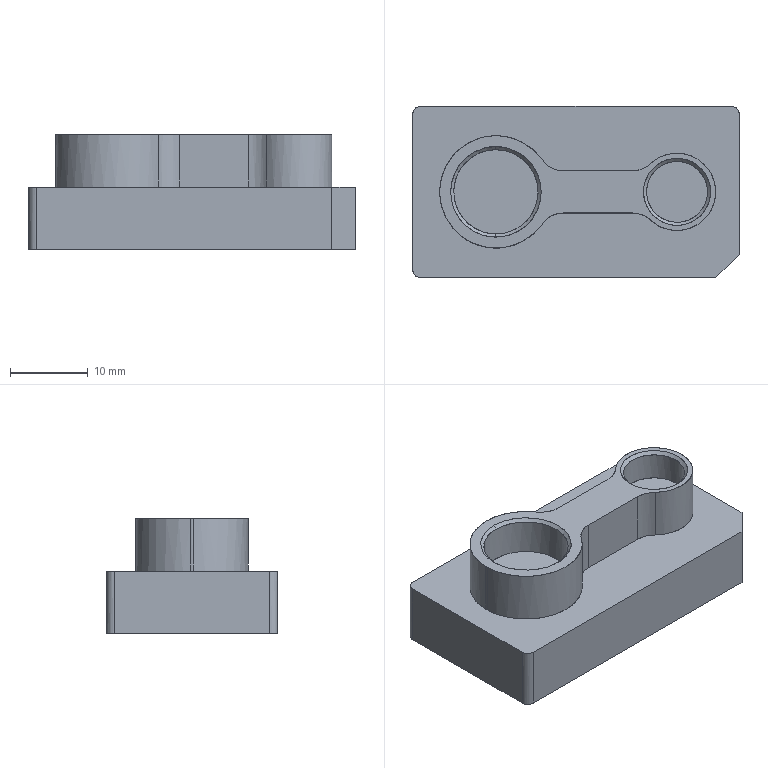NC program | PowerMill | posted by the shop | part box 42 x 22 x 14.721 mm
Lines 1 to 1508 of 84704:
%
G40 G49 G17 G80
( TOOL ID   D10C_1_1 )
( TOOL DIA. 10. TIP RAD 0 LENGTH 70.16 )
( Z = -.069 )
T1 M6
T2
G91 G28 Z0
G0 G90 G54
M08
S8000 M3
G0 X0 Y0 M8
G43 Z10.2 H1
X28.78 Y13.78
Z1.131
G1 Z-.069 F6000
X23.78 F10000
X-23.78
Y8.268
X23.78
Y2.756
X-23.78
Y-2.756
X23.78
Y-8.268
X-23.78
Y-13.78
X23.78
X28.78
G0 Z10.2
X.211 Y.009
Z9.881
X31.026 Y4.95
Z.692
G1 Z-.508 F6000
X30.499 F10000
G3 X25.751 Y.202 I0 J-4.747
G1 Y-14.007
G2 X24.751 Y-15.007 I-1. J0
G1 X-24.329
G2 X-25.329 Y-14.007 I0 J1.
G1 Y14.024
G2 X-24.329 Y15.024 I1. J0
G1 X24.751
G2 X25.751 Y14.024 I0 J-1.
G1 Y.202
X23.249 Y.105
X23.253 Y.009
X23.224 Y-.765
X23.136 Y-1.538
X22.988 Y-2.312
X22.777 Y-3.085
X22.497 Y-3.859
X22.147 Y-4.632
X21.867 Y-5.145
X21.182 Y-6.179
X20.32 Y-7.179
X19.547 Y-7.885
X18.773 Y-8.463
X18. Y-8.949
X17.226 Y-9.333
X16.453 Y-9.653
X15.68 Y-9.894
X15.033 Y-10.046
X14.133 Y-10.189
X13.359 Y-10.245
X12.586 Y-10.243
X11.812 Y-10.182
X11.039 Y-10.063
X10.266 Y-9.879
X9.492 Y-9.634
X8.719 Y-9.315
X7.945 Y-8.916
X7.266 Y-8.499
X6.727 Y-8.093
X6.585 Y-8.019
X6.427 Y-7.993
X-.452
G3 X-.828 Y-8.163 I0 J-.5
G1 X-1.123 Y-8.499
X-1.91 Y-9.273
X-2.849 Y-10.046
X-3.656 Y-10.599
X-4.029 Y-10.819
X-5.203 Y-11.421
X-5.976 Y-11.737
X-6.75 Y-11.987
X-7.523 Y-12.2
X-8.443 Y-12.366
X-9.07 Y-12.45
X-9.844 Y-12.499
X-10.617 Y-12.506
X-11.39 Y-12.465
X-12.164 Y-12.371
X-12.937 Y-12.23
X-13.711 Y-12.037
X-15.012 Y-11.593
X-16.031 Y-11.122
X-16.584 Y-10.819
X-17.578 Y-10.177
X-18.351 Y-9.581
X-18.696 Y-9.273
X-19.487 Y-8.499
X-20.144 Y-7.726
X-20.672 Y-6.988
X-21.185 Y-6.179
X-21.588 Y-5.405
X-21.925 Y-4.632
X-22.206 Y-3.859
X-22.427 Y-3.085
X-22.594 Y-2.312
X-22.722 Y-1.538
X-22.83 Y.009
X-22.719 Y1.555
X-22.594 Y2.329
X-22.421 Y3.102
X-22.218 Y3.825
X-21.917 Y4.649
X-21.572 Y5.422
X-21.175 Y6.196
X-20.687 Y6.969
X-20.133 Y7.743
X-19.469 Y8.516
X-18.687 Y9.29
X-17.739 Y10.063
X-16.56 Y10.836
X-15.258 Y11.491
X-14.961 Y11.61
X-13.711 Y12.04
X-12.937 Y12.233
X-12.099 Y12.383
X-10.617 Y12.516
X-9.844 Y12.505
X-8.511 Y12.383
X-7.523 Y12.2
X-6.75 Y11.989
X-5.639 Y11.61
X-4.43 Y11.048
X-3.656 Y10.598
X-2.883 Y10.071
X-2.109 Y9.454
X-1.336 Y8.712
X-.829 Y8.156
G3 X-.46 Y7.993 I.37 J.337
G1 X6.424
X6.584 Y8.019
X6.727 Y8.095
X7.172 Y8.435
X7.945 Y8.916
X8.663 Y9.29
X9.492 Y9.634
X10.266 Y9.879
X11.04 Y10.063
X11.812 Y10.182
X12.586 Y10.243
X13.359 Y10.245
X14.133 Y10.188
X14.906 Y10.073
X15.68 Y9.894
X16.453 Y9.653
X17.226 Y9.333
X18. Y8.949
X18.773 Y8.463
X19.547 Y7.885
X20.32 Y7.179
X21.094 Y6.292
X21.69 Y5.422
X22.138 Y4.649
X22.49 Y3.876
X22.772 Y3.102
X22.984 Y2.329
X23.134 Y1.555
X23.223 Y.782
X23.249 Y.105
X25.751 Y.202
G0 Z3.303
G1 X31.026 Y4.95
G0 Z.303
G1 Z-.897 F6000
X30.499 F10000
G3 X25.751 Y.202 I0 J-4.747
G1 Y-14.007
G2 X24.751 Y-15.007 I-1. J0
G1 X-24.329
G2 X-25.329 Y-14.007 I0 J1.
G1 Y14.024
G2 X-24.329 Y15.024 I1. J0
G1 X24.751
G2 X25.751 Y14.024 I0 J-1.
G1 Y.202
X23.249 Y.105
X23.253 Y.009
X23.224 Y-.765
X23.137 Y-1.538
X22.988 Y-2.312
X22.777 Y-3.085
X22.497 Y-3.859
X22.147 Y-4.632
X21.867 Y-5.145
X21.182 Y-6.179
X20.32 Y-7.179
X19.547 Y-7.885
X18.773 Y-8.463
X18. Y-8.949
X17.226 Y-9.333
X16.453 Y-9.653
X15.68 Y-9.894
X15.033 Y-10.046
X14.133 Y-10.189
X13.359 Y-10.245
X12.586 Y-10.243
X11.812 Y-10.182
X11.039 Y-10.063
X10.266 Y-9.879
X9.492 Y-9.634
X8.719 Y-9.315
X7.945 Y-8.916
X7.266 Y-8.499
X6.727 Y-8.093
X6.585 Y-8.019
X6.427 Y-7.993
X-.452
G3 X-.828 Y-8.163 I0 J-.5
G1 X-1.123 Y-8.499
X-1.91 Y-9.273
X-2.849 Y-10.046
X-3.656 Y-10.599
X-4.029 Y-10.819
X-5.203 Y-11.421
X-5.976 Y-11.737
X-6.75 Y-11.987
X-7.523 Y-12.2
X-8.443 Y-12.366
X-9.07 Y-12.45
X-9.844 Y-12.499
X-10.617 Y-12.506
X-11.39 Y-12.465
X-12.164 Y-12.371
X-12.937 Y-12.23
X-13.711 Y-12.037
X-15.012 Y-11.593
X-16.031 Y-11.122
X-16.584 Y-10.819
X-17.578 Y-10.177
X-18.351 Y-9.581
X-18.696 Y-9.273
X-19.487 Y-8.499
X-20.144 Y-7.726
X-20.672 Y-6.988
X-21.185 Y-6.179
X-21.588 Y-5.405
X-21.925 Y-4.632
X-22.206 Y-3.859
X-22.427 Y-3.085
X-22.594 Y-2.312
X-22.722 Y-1.538
X-22.83 Y.009
X-22.719 Y1.555
X-22.594 Y2.329
X-22.421 Y3.102
X-22.218 Y3.825
X-21.917 Y4.649
X-21.572 Y5.422
X-21.176 Y6.196
X-20.687 Y6.969
X-20.133 Y7.743
X-19.469 Y8.516
X-18.687 Y9.29
X-17.739 Y10.063
X-16.56 Y10.836
X-15.258 Y11.491
X-14.961 Y11.61
X-13.711 Y12.04
X-12.937 Y12.233
X-12.099 Y12.383
X-10.617 Y12.516
X-9.844 Y12.505
X-8.511 Y12.383
X-7.523 Y12.2
X-6.75 Y11.989
X-5.639 Y11.61
X-4.43 Y11.048
X-3.656 Y10.598
X-2.883 Y10.071
X-2.109 Y9.454
X-1.336 Y8.712
X-.829 Y8.156
G3 X-.46 Y7.993 I.37 J.337
G1 X6.424
X6.584 Y8.019
X6.727 Y8.095
X7.172 Y8.435
X7.945 Y8.916
X8.663 Y9.29
X9.492 Y9.634
X10.266 Y9.879
X11.04 Y10.063
X11.812 Y10.182
X12.586 Y10.243
X13.359 Y10.245
X14.133 Y10.188
X14.906 Y10.073
X15.68 Y9.894
X16.453 Y9.653
X17.226 Y9.333
X18. Y8.949
X18.773 Y8.463
X19.547 Y7.885
X20.32 Y7.179
X21.094 Y6.292
X21.69 Y5.422
X22.138 Y4.649
X22.49 Y3.876
X22.772 Y3.102
X22.984 Y2.329
X23.134 Y1.555
X23.223 Y.782
X23.249 Y.105
X25.751 Y.202
G0 Z2.914
G1 X31.026 Y4.95
G0 Z-.086
G1 Z-1.286 F6000
X30.499 F10000
G3 X25.751 Y.202 I0 J-4.747
G1 Y-14.007
G2 X24.751 Y-15.007 I-1. J0
G1 X-24.329
G2 X-25.329 Y-14.007 I0 J1.
G1 Y14.024
G2 X-24.329 Y15.024 I1. J0
G1 X24.751
G2 X25.751 Y14.024 I0 J-1.
G1 Y.202
X23.249 Y.105
X23.253 Y.009
X23.224 Y-.765
X23.137 Y-1.538
X22.988 Y-2.312
X22.777 Y-3.085
X22.497 Y-3.859
X22.147 Y-4.632
X21.867 Y-5.145
X21.182 Y-6.179
X20.32 Y-7.179
X19.547 Y-7.885
X18.773 Y-8.463
X18. Y-8.949
X17.226 Y-9.333
X16.453 Y-9.653
X15.68 Y-9.894
X15.664 Y-9.897
X15.033 Y-10.046
X15.002 Y-10.051
X14.906 Y-10.073
X14.133 Y-10.189
X13.359 Y-10.245
X12.586 Y-10.243
X11.812 Y-10.182
X11.039 Y-10.063
X10.266 Y-9.879
X9.492 Y-9.634
X8.719 Y-9.315
X7.945 Y-8.916
X7.266 Y-8.499
X6.727 Y-8.093
X6.585 Y-8.019
X6.427 Y-7.993
X-.452
G3 X-.828 Y-8.163 I0 J-.5
G1 X-1.123 Y-8.499
X-1.91 Y-9.273
X-2.849 Y-10.046
X-3.656 Y-10.599
X-4.029 Y-10.819
X-5.203 Y-11.421
X-5.976 Y-11.737
X-6.75 Y-11.987
X-7.523 Y-12.2
X-8.443 Y-12.366
X-9.07 Y-12.45
X-9.844 Y-12.499
X-10.617 Y-12.506
X-11.39 Y-12.465
X-12.164 Y-12.371
X-12.937 Y-12.23
X-13.711 Y-12.037
X-15.012 Y-11.593
X-16.031 Y-11.122
X-16.584 Y-10.819
X-17.578 Y-10.177
X-18.351 Y-9.581
X-18.696 Y-9.273
X-19.487 Y-8.499
X-20.144 Y-7.726
X-20.672 Y-6.988
X-21.185 Y-6.179
X-21.588 Y-5.405
X-21.925 Y-4.632
X-22.206 Y-3.859
X-22.427 Y-3.085
X-22.594 Y-2.312
X-22.722 Y-1.538
X-22.83 Y.009
X-22.719 Y1.555
X-22.594 Y2.329
X-22.421 Y3.102
X-22.218 Y3.825
X-21.917 Y4.649
X-21.572 Y5.422
X-21.176 Y6.196
X-20.687 Y6.969
X-20.133 Y7.743
X-19.469 Y8.516
X-18.687 Y9.29
X-17.739 Y10.063
X-16.56 Y10.836
X-15.258 Y11.491
X-14.961 Y11.61
X-13.711 Y12.04
X-12.937 Y12.233
X-12.099 Y12.383
X-10.617 Y12.516
X-9.844 Y12.505
X-8.511 Y12.383
X-7.523 Y12.2
X-6.75 Y11.989
X-5.639 Y11.61
X-4.43 Y11.048
X-3.656 Y10.598
X-2.883 Y10.071
X-2.109 Y9.454
X-1.336 Y8.712
X-.829 Y8.156
G3 X-.46 Y7.993 I.37 J.337
G1 X6.424
X6.584 Y8.019
X6.727 Y8.095
X7.172 Y8.435
X7.945 Y8.916
X8.663 Y9.29
X9.492 Y9.634
X10.266 Y9.879
X11.04 Y10.063
X11.812 Y10.182
X12.586 Y10.243
X13.359 Y10.245
X14.133 Y10.188
X14.906 Y10.073
X15.68 Y9.894
X16.453 Y9.653
X17.226 Y9.333
X18. Y8.949
X18.773 Y8.463
X19.547 Y7.885
X20.32 Y7.179
X21.094 Y6.292
X21.69 Y5.422
X22.138 Y4.649
X22.49 Y3.876
X22.772 Y3.102
X22.984 Y2.329
X23.134 Y1.555
X23.223 Y.782
X23.249 Y.105
X25.751 Y.202
G0 Z2.525
G1 X31.026 Y4.95
G0 Z-.475
G1 Z-1.675 F6000
X30.499 F10000
G3 X25.751 Y.202 I0 J-4.747
G1 Y-14.007
G2 X24.751 Y-15.007 I-1. J0
G1 X-24.329
G2 X-25.329 Y-14.007 I0 J1.
G1 Y14.024
G2 X-24.329 Y15.024 I1. J0
G1 X24.751
G2 X25.751 Y14.024 I0 J-1.
G1 Y.202
X23.249 Y.105
X23.253 Y.009
X23.224 Y-.765
X23.137 Y-1.538
X22.988 Y-2.312
X22.777 Y-3.085
X22.497 Y-3.859
X22.147 Y-4.632
X21.867 Y-5.145
X21.182 Y-6.179
X20.32 Y-7.179
X19.547 Y-7.885
X18.773 Y-8.463
X18. Y-8.949
X17.226 Y-9.333
X16.453 Y-9.653
X15.68 Y-9.894
X15.648 Y-9.901
X15.033 Y-10.046
X15.003 Y-10.051
X14.906 Y-10.073
X14.133 Y-10.189
X13.359 Y-10.245
X12.586 Y-10.243
X11.812 Y-10.182
X11.039 Y-10.063
X10.266 Y-9.879
X9.492 Y-9.634
X8.719 Y-9.315
X7.945 Y-8.916
X7.266 Y-8.499
X6.727 Y-8.093
X6.585 Y-8.019
X6.427 Y-7.993
X-.452
G3 X-.828 Y-8.163 I0 J-.5
G1 X-1.123 Y-8.499
X-1.91 Y-9.273
X-2.849 Y-10.046
X-3.656 Y-10.599
X-4.029 Y-10.819
X-5.203 Y-11.421
X-5.976 Y-11.737
X-6.75 Y-11.987
X-7.523 Y-12.2
X-8.443 Y-12.366
X-9.07 Y-12.45
X-9.844 Y-12.499
X-10.617 Y-12.506
X-11.39 Y-12.465
X-12.164 Y-12.371
X-12.937 Y-12.23
X-13.711 Y-12.037
X-15.012 Y-11.593
X-16.031 Y-11.122
X-16.584 Y-10.819
X-17.578 Y-10.178
X-18.351 Y-9.581
X-18.696 Y-9.273
X-19.487 Y-8.499
X-20.144 Y-7.726
X-20.672 Y-6.988
X-21.185 Y-6.179
X-21.588 Y-5.405
X-21.925 Y-4.632
X-22.206 Y-3.859
X-22.427 Y-3.085
X-22.594 Y-2.312
X-22.722 Y-1.538
X-22.83 Y.009
X-22.719 Y1.555
X-22.594 Y2.329
X-22.421 Y3.102
X-22.218 Y3.825
X-21.917 Y4.649
X-21.572 Y5.422
X-21.176 Y6.196
X-20.687 Y6.969
X-20.133 Y7.743
X-19.469 Y8.516
X-18.687 Y9.29
X-17.739 Y10.063
X-16.56 Y10.836
X-15.258 Y11.491
X-14.961 Y11.61
X-13.711 Y12.04
X-12.937 Y12.233
X-12.099 Y12.383
X-10.617 Y12.516
X-9.844 Y12.505
X-8.511 Y12.383
X-7.523 Y12.2
X-6.75 Y11.989
X-5.639 Y11.61
X-4.43 Y11.048
X-3.656 Y10.598
X-2.883 Y10.071
X-2.109 Y9.454
X-1.336 Y8.712
X-.829 Y8.156
G3 X-.46 Y7.993 I.37 J.337
G1 X6.424
X6.584 Y8.019
X6.727 Y8.095
X7.172 Y8.435
X7.945 Y8.916
X8.663 Y9.29
X9.492 Y9.634
X10.266 Y9.879
X11.04 Y10.063
X11.812 Y10.182
X12.586 Y10.243
X13.359 Y10.245
X14.133 Y10.188
X14.906 Y10.073
X15.68 Y9.894
X16.453 Y9.653
X17.226 Y9.333
X18. Y8.949
X18.773 Y8.463
X19.547 Y7.885
X20.32 Y7.179
X21.094 Y6.292
X21.69 Y5.422
X22.138 Y4.649
X22.49 Y3.876
X22.772 Y3.102
X22.984 Y2.329
X23.134 Y1.555
X23.223 Y.782
X23.249 Y.105
X25.751 Y.202
G0 Z2.137
G1 X31.026 Y4.95
G0 Z-.863
G1 Z-2.063 F6000
X30.499 F10000
G3 X25.751 Y.202 I0 J-4.747
G1 Y-14.007
G2 X24.751 Y-15.007 I-1. J0
G1 X-24.329
G2 X-25.329 Y-14.007 I0 J1.
G1 Y14.024
G2 X-24.329 Y15.024 I1. J0
G1 X24.751
G2 X25.751 Y14.024 I0 J-1.
G1 Y.202
X23.249 Y.105
X23.253 Y.009
X23.224 Y-.765
X23.137 Y-1.538
X22.988 Y-2.312
X22.777 Y-3.085
X22.497 Y-3.859
X22.147 Y-4.632
X21.867 Y-5.145
X21.182 Y-6.179
X20.32 Y-7.179
X19.547 Y-7.885
X18.773 Y-8.463
X18. Y-8.949
X17.226 Y-9.333
X16.453 Y-9.653
X15.68 Y-9.894
X15.632 Y-9.905
X15.033 Y-10.046
X15.004 Y-10.05
X14.906 Y-10.073
X14.133 Y-10.189
X13.359 Y-10.245
X12.586 Y-10.243
X11.812 Y-10.182
X11.039 Y-10.063
X10.266 Y-9.879
X9.492 Y-9.634
X8.719 Y-9.315
X7.945 Y-8.916
X7.266 Y-8.499
X6.727 Y-8.093
X6.585 Y-8.019
X6.427 Y-7.993
X-.452
G3 X-.828 Y-8.163 I0 J-.5
G1 X-1.123 Y-8.499
X-1.91 Y-9.273
X-2.849 Y-10.046
X-3.656 Y-10.599
X-4.029 Y-10.819
X-5.203 Y-11.421
X-5.976 Y-11.737
X-6.75 Y-11.987
X-7.523 Y-12.2
X-8.443 Y-12.366
X-9.07 Y-12.45
X-9.844 Y-12.499
X-10.617 Y-12.506
X-11.39 Y-12.465
X-12.164 Y-12.371
X-12.937 Y-12.23
X-13.711 Y-12.037
X-15.012 Y-11.593
X-16.031 Y-11.122
X-16.584 Y-10.819
X-17.578 Y-10.178
X-18.351 Y-9.581
X-18.696 Y-9.273
X-19.487 Y-8.499
X-20.144 Y-7.726
X-20.672 Y-6.988
X-21.185 Y-6.179
X-21.588 Y-5.405
X-21.925 Y-4.632
X-22.206 Y-3.859
X-22.427 Y-3.085
X-22.594 Y-2.312
X-22.722 Y-1.538
X-22.83 Y.009
X-22.719 Y1.555
X-22.594 Y2.329
X-22.421 Y3.102
X-22.218 Y3.825
X-21.917 Y4.649
X-21.572 Y5.422
X-21.176 Y6.196
X-20.687 Y6.969
X-20.133 Y7.743
X-19.469 Y8.516
X-18.687 Y9.29
X-17.739 Y10.063
X-16.56 Y10.836
X-15.258 Y11.491
X-14.961 Y11.61
X-13.711 Y12.04
X-12.937 Y12.233
X-12.099 Y12.383
X-10.617 Y12.516
X-9.844 Y12.505
X-8.511 Y12.383
X-7.523 Y12.2
X-6.75 Y11.989
X-5.639 Y11.61
X-4.43 Y11.048
X-3.656 Y10.598
X-2.883 Y10.071
X-2.109 Y9.454
X-1.336 Y8.712
X-.829 Y8.156
G3 X-.46 Y7.993 I.37 J.337
G1 X6.424
X6.584 Y8.019
X6.727 Y8.095
X7.172 Y8.435
X7.945 Y8.916
X8.663 Y9.29
X9.492 Y9.634
X10.266 Y9.879
X11.04 Y10.063
X11.812 Y10.182
X12.586 Y10.243
X13.359 Y10.245
X14.133 Y10.188
X14.906 Y10.073
X15.68 Y9.894
X16.453 Y9.653
X17.226 Y9.333
X18. Y8.949
X18.773 Y8.463
X19.547 Y7.885
X20.32 Y7.179
X21.094 Y6.292
X21.69 Y5.422
X22.138 Y4.649
X22.49 Y3.876
X22.772 Y3.102
X22.984 Y2.329
X23.134 Y1.555
X23.223 Y.782
X23.249 Y.105
X25.751 Y.202
G0 Z1.748
G1 X31.026 Y4.95
G0 Z-1.252
G1 Z-2.452 F6000
X30.499 F10000
G3 X25.751 Y.202 I0 J-4.747
G1 Y-14.007
G2 X24.751 Y-15.007 I-1. J0
G1 X-24.329
G2 X-25.329 Y-14.007 I0 J1.
G1 Y14.024
G2 X-24.329 Y15.024 I1. J0
G1 X24.751
G2 X25.751 Y14.024 I0 J-1.
G1 Y.202
X23.249 Y.105
X23.253 Y.009
X23.224 Y-.765
X23.137 Y-1.538
X22.989 Y-2.312
X22.777 Y-3.085
X22.497 Y-3.859
X22.147 Y-4.632
X21.867 Y-5.145
X21.182 Y-6.179
X20.32 Y-7.179
X19.547 Y-7.885
X18.773 Y-8.463
X18. Y-8.949
X17.226 Y-9.333
X16.453 Y-9.653
X15.68 Y-9.894
X15.616 Y-9.909
X15.033 Y-10.046
X15.005 Y-10.05
X14.906 Y-10.073
X14.133 Y-10.189
X13.359 Y-10.245
X12.586 Y-10.243
X11.812 Y-10.182
X11.039 Y-10.063
X10.266 Y-9.879
X9.492 Y-9.634
X8.719 Y-9.315
X7.945 Y-8.916
X7.266 Y-8.499
X6.727 Y-8.093
X6.585 Y-8.019
X6.427 Y-7.993
X-.452
G3 X-.828 Y-8.163 I0 J-.5
G1 X-1.123 Y-8.499
X-1.91 Y-9.273
X-2.849 Y-10.046
X-3.656 Y-10.599
X-4.029 Y-10.819
X-5.203 Y-11.421
X-5.976 Y-11.737
X-6.75 Y-11.987
X-7.523 Y-12.2
X-8.443 Y-12.366
X-9.07 Y-12.45
X-9.844 Y-12.499
X-10.617 Y-12.506
X-11.39 Y-12.465
X-12.164 Y-12.371
X-12.937 Y-12.23
X-13.711 Y-12.037
X-15.012 Y-11.593
X-16.031 Y-11.122
X-16.584 Y-10.819
X-17.578 Y-10.178
X-18.351 Y-9.581
X-18.696 Y-9.273
X-19.487 Y-8.499
X-20.144 Y-7.726
X-20.672 Y-6.988
X-21.185 Y-6.179
X-21.588 Y-5.405
X-21.925 Y-4.632
X-22.206 Y-3.859
X-22.427 Y-3.085
X-22.594 Y-2.312
X-22.722 Y-1.538
X-22.83 Y.009
X-22.719 Y1.555
X-22.594 Y2.329
X-22.421 Y3.102
X-22.218 Y3.825
X-21.917 Y4.649
X-21.573 Y5.422
X-21.176 Y6.196
X-20.687 Y6.969
X-20.133 Y7.743
X-19.469 Y8.516
X-18.687 Y9.29
X-17.739 Y10.063
X-16.56 Y10.836
X-15.258 Y11.491
X-14.961 Y11.61
X-13.711 Y12.04
X-12.937 Y12.233
X-12.099 Y12.383
X-10.617 Y12.516
X-9.844 Y12.505
X-8.511 Y12.383
X-7.523 Y12.2
X-6.75 Y11.989
X-5.639 Y11.61
X-4.43 Y11.048
X-3.656 Y10.598
X-2.883 Y10.071
X-2.109 Y9.454
X-1.336 Y8.712
X-.829 Y8.156
G3 X-.46 Y7.993 I.37 J.337
G1 X6.424
X6.584 Y8.019
X6.727 Y8.095
X7.172 Y8.435
X7.945 Y8.916
X8.663 Y9.29
X9.492 Y9.634
X10.266 Y9.879
X11.039 Y10.063
X11.04
X11.045 Y10.064
X11.812 Y10.182
X12.586 Y10.243
X13.359 Y10.245
X14.133 Y10.188
X14.906 Y10.073
X15.68 Y9.894
X16.453 Y9.653
X17.226 Y9.333
X18. Y8.949
X18.773 Y8.463
X19.547 Y7.885
X20.32 Y7.179
X21.094 Y6.292
X21.69 Y5.422
X22.138 Y4.649
X22.49 Y3.876
X22.772 Y3.102
X22.984 Y2.329
X23.134 Y1.555
X23.223 Y.782
X23.249 Y.105
X25.751 Y.202
G0 Z1.359
G1 X31.026 Y4.95
G0 Z-1.641
G1 Z-2.841 F6000
X30.499 F10000
G3 X25.751 Y.202 I0 J-4.747
G1 Y-14.007
G2 X24.751 Y-15.007 I-1. J0
G1 X-24.329
G2 X-25.329 Y-14.007 I0 J1.
G1 Y14.024
G2 X-24.329 Y15.024 I1. J0
G1 X24.751
G2 X25.751 Y14.024 I0 J-1.
G1 Y.202
X23.249 Y.105
X23.253 Y.009
X23.224 Y-.765
X23.137 Y-1.538
X22.989 Y-2.312
X22.777 Y-3.085
X22.497 Y-3.859
X22.147 Y-4.632
X21.867 Y-5.145
X21.182 Y-6.179
X20.32 Y-7.179
X19.547 Y-7.885
X18.773 Y-8.463
X18. Y-8.949
X17.226 Y-9.333
X16.453 Y-9.653
X15.68 Y-9.894
X15.6 Y-9.912
X15.033 Y-10.046
X15.005 Y-10.05
X14.906 Y-10.073
X14.133 Y-10.189
X13.359 Y-10.245
X12.586 Y-10.243
X11.812 Y-10.182
X11.039 Y-10.063
X10.266 Y-9.879
X9.492 Y-9.634
X8.719 Y-9.315
X7.945 Y-8.916
X7.266 Y-8.499
X6.727 Y-8.093
X6.585 Y-8.019
X6.427 Y-7.993
X-.452
G3 X-.828 Y-8.163 I0 J-.5
G1 X-1.123 Y-8.499
X-1.91 Y-9.273
X-2.849 Y-10.046
X-3.656 Y-10.599
X-4.029 Y-10.819
X-5.203 Y-11.421
X-5.976 Y-11.737
X-6.75 Y-11.987
X-7.523 Y-12.2
X-8.443 Y-12.366
X-9.07 Y-12.45
X-9.844 Y-12.499
X-10.617 Y-12.506
X-11.39 Y-12.465
X-12.164 Y-12.371
X-12.937 Y-12.23
X-13.711 Y-12.037
X-15.012 Y-11.593
X-16.031 Y-11.122
X-16.584 Y-10.819
X-17.578 Y-10.178
X-18.351 Y-9.581
X-18.696 Y-9.273
X-19.487 Y-8.499
X-20.144 Y-7.726
X-20.672 Y-6.988
X-21.185 Y-6.179
X-21.588 Y-5.405
X-21.925 Y-4.632
X-22.206 Y-3.859
X-22.427 Y-3.085
X-22.594 Y-2.312
X-22.722 Y-1.538
X-22.83 Y.009
X-22.719 Y1.555
X-22.594 Y2.329
X-22.421 Y3.102
X-22.218 Y3.825
X-21.917 Y4.649
X-21.573 Y5.422
X-21.176 Y6.196
X-20.687 Y6.969
X-20.133 Y7.743
X-19.469 Y8.516
X-18.687 Y9.29
X-17.739 Y10.063
X-16.56 Y10.836
X-15.258 Y11.491
X-14.961 Y11.61
X-13.711 Y12.04
X-12.937 Y12.233
X-12.099 Y12.383
X-10.617 Y12.516
X-9.844 Y12.505
X-8.511 Y12.383
X-7.523 Y12.2
X-6.75 Y11.989
X-5.639 Y11.61
X-4.43 Y11.048
X-3.656 Y10.598
X-2.883 Y10.071
X-2.109 Y9.454
X-1.336 Y8.712
X-.829 Y8.156
G3 X-.46 Y7.993 I.37 J.337
G1 X6.424
X6.584 Y8.019
X6.727 Y8.095
X7.172 Y8.435
X7.945 Y8.916
X8.663 Y9.29
X9.492 Y9.634
X10.266 Y9.879
X11.039 Y10.063
X11.812 Y10.182
X12.586 Y10.243
X13.359 Y10.245
X14.133 Y10.188
X14.906 Y10.073
X15.68 Y9.894
X16.453 Y9.653
X17.226 Y9.333
X18. Y8.949
X18.773 Y8.463
X19.547 Y7.885
X20.32 Y7.179
X21.094 Y6.292
X21.69 Y5.422
X22.138 Y4.649
X22.49 Y3.876
X22.772 Y3.102
X22.984 Y2.329
X23.134 Y1.555
X23.223 Y.782
X23.249 Y.105
X25.751 Y.202
G0 Z.97
G1 X31.026 Y4.95
G0 Z-2.03
G1 Z-3.23 F6000
X30.499 F10000
G3 X25.751 Y.202 I0 J-4.747
G1 Y-14.007
G2 X24.751 Y-15.007 I-1. J0
G1 X-24.329
G2 X-25.329 Y-14.007 I0 J1.
G1 Y14.024
G2 X-24.329 Y15.024 I1. J0
G1 X24.751
G2 X25.751 Y14.024 I0 J-1.
G1 Y.202
X23.249 Y.105
X23.253 Y.009
X23.224 Y-.765
X23.137 Y-1.538
X22.989 Y-2.312
X22.777 Y-3.085
X22.497 Y-3.859
X22.147 Y-4.632
X21.867 Y-5.145
X21.182 Y-6.179
X20.32 Y-7.179
X19.547 Y-7.885
X18.773 Y-8.463
X18. Y-8.949
X17.226 Y-9.333
X16.453 Y-9.653
X15.68 Y-9.894
X15.584 Y-9.916
X15.033 Y-10.046
X15.006 Y-10.05
X14.906 Y-10.073
X14.133 Y-10.189
X13.359 Y-10.245
X12.586 Y-10.243
X11.812 Y-10.182
X11.039 Y-10.063
X10.266 Y-9.879
X9.492 Y-9.634
X8.719 Y-9.315
X7.945 Y-8.916
X7.266 Y-8.499
X6.727 Y-8.093
X6.585 Y-8.019
X6.427 Y-7.993
X-.452
G3 X-.828 Y-8.163 I0 J-.5
G1 X-1.123 Y-8.499
X-1.91 Y-9.273
X-2.849 Y-10.046
X-3.656 Y-10.599
X-4.029 Y-10.819
X-5.203 Y-11.421
X-5.976 Y-11.737
X-6.75 Y-11.987
X-7.523 Y-12.2
X-8.443 Y-12.366
X-9.07 Y-12.45
X-9.844 Y-12.499
X-10.617 Y-12.506
X-11.39 Y-12.465
X-12.164 Y-12.371
X-12.937 Y-12.23
X-13.711 Y-12.037
X-15.012 Y-11.593
X-16.031 Y-11.122
X-16.584 Y-10.819
X-17.578 Y-10.178
X-18.351 Y-9.582
X-18.696 Y-9.273
X-19.487 Y-8.499
X-20.144 Y-7.726
X-20.672 Y-6.988
X-21.185 Y-6.179
X-21.588 Y-5.405
X-21.925 Y-4.632
X-22.206 Y-3.859
X-22.427 Y-3.085
X-22.594 Y-2.312
X-22.722 Y-1.538
X-22.83 Y.009
X-22.719 Y1.555
X-22.594 Y2.329
X-22.421 Y3.102
X-22.218 Y3.825
X-21.917 Y4.649
X-21.573 Y5.422
X-21.176 Y6.196
X-20.687 Y6.969
X-20.133 Y7.743
X-19.469 Y8.516
X-18.687 Y9.29
X-17.739 Y10.063
X-16.56 Y10.836
X-15.258 Y11.491
X-14.961 Y11.61
X-13.711 Y12.04
X-12.937 Y12.233
X-12.164 Y12.374
X-12.139 Y12.376
X-12.099 Y12.383
X-10.641 Y12.514
X-10.617 Y12.516
X-9.844 Y12.505
X-8.511 Y12.383
X-7.523 Y12.2
X-6.75 Y11.989
X-5.639 Y11.61
X-4.43 Y11.048
X-3.656 Y10.598
X-2.883 Y10.071
X-2.109 Y9.454
X-1.336 Y8.712
X-.829 Y8.156
G3 X-.46 Y7.993 I.37 J.337
G1 X6.424
X6.584 Y8.019
X6.727 Y8.095
X7.172 Y8.435
X7.945 Y8.916
X8.663 Y9.29
X9.492 Y9.634
X10.266 Y9.879
X11.039 Y10.063
X11.812 Y10.182
X12.586 Y10.243
X13.359 Y10.245
X14.133 Y10.188
X14.906 Y10.073
X15.68 Y9.894
X16.453 Y9.653
X17.226 Y9.333
X18. Y8.949
X18.773 Y8.463
X19.547 Y7.885
X20.32 Y7.179
X21.094 Y6.292
X21.69 Y5.422
X22.138 Y4.649
X22.49 Y3.876
X22.772 Y3.102
X22.984 Y2.329
X23.134 Y1.555
X23.223 Y.782
X23.249 Y.105
X25.751 Y.202
G0 Z.581
G1 X31.026 Y4.95
G0 Z-2.419
G1 Z-3.619 F6000
X30.499 F10000
G3 X25.751 Y.202 I0 J-4.747
G1 Y-14.007
G2 X24.751 Y-15.007 I-1. J0
G1 X-24.329
G2 X-25.329 Y-14.007 I0 J1.
G1 Y14.024
G2 X-24.329 Y15.024 I1. J0
G1 X24.751
G2 X25.751 Y14.024 I0 J-1.
G1 Y.202
X23.249 Y.105
X23.253 Y.009
X23.224 Y-.765
X23.137 Y-1.538
X22.989 Y-2.312
X22.777 Y-3.085
X22.497 Y-3.859
X22.147 Y-4.632
X21.867 Y-5.145
X21.182 Y-6.179
X20.32 Y-7.179
X19.547 Y-7.885
X18.773 Y-8.463
X18. Y-8.949
X17.226 Y-9.333
X16.453 Y-9.653
X15.68 Y-9.894
X15.568 Y-9.92
X15.033 Y-10.046
X15.007 Y-10.05
X14.906 Y-10.073
X14.133 Y-10.189
X13.359 Y-10.245
X12.586 Y-10.243
X11.812 Y-10.182
X11.039 Y-10.063
X10.266 Y-9.879
X9.492 Y-9.634
X8.719 Y-9.315
X7.945 Y-8.916
X7.266 Y-8.499
X6.727 Y-8.093
X6.585 Y-8.019
X6.427 Y-7.993
X-.452
G3 X-.828 Y-8.163 I0 J-.5
G1 X-1.123 Y-8.499
X-1.91 Y-9.273
X-2.849 Y-10.046
X-3.656 Y-10.599
X-4.029 Y-10.819
X-5.203 Y-11.421
X-5.976 Y-11.737
X-6.75 Y-11.987
X-7.523 Y-12.2
X-8.443 Y-12.366
X-9.07 Y-12.45
X-9.844 Y-12.499
X-10.617 Y-12.506
X-11.39 Y-12.465
X-12.164 Y-12.371
X-12.937 Y-12.23
X-13.711 Y-12.037
X-15.012 Y-11.593
X-16.031 Y-11.122
X-16.584 Y-10.819
X-17.578 Y-10.178
X-18.351 Y-9.582
X-18.696 Y-9.273
X-19.487 Y-8.499
X-20.144 Y-7.726
X-20.672 Y-6.988
X-21.185 Y-6.179
X-21.588 Y-5.405
X-21.925 Y-4.632
X-22.206 Y-3.859
X-22.427 Y-3.085
X-22.594 Y-2.312
X-22.722 Y-1.538
X-22.83 Y.009
X-22.719 Y1.555
X-22.594 Y2.329
X-22.421 Y3.102
X-22.218 Y3.825
X-21.917 Y4.649
X-21.573 Y5.422
X-21.176 Y6.196
X-20.687 Y6.969
X-20.133 Y7.743
X-19.469 Y8.516
X-18.687 Y9.29
X-17.739 Y10.063
X-16.56 Y10.836
X-15.258 Y11.491
X-14.961 Y11.61
X-13.711 Y12.04
X-12.937 Y12.233
X-12.164 Y12.374
X-12.138 Y12.376
X-12.099 Y12.383
X-10.664 Y12.512
X-10.617 Y12.516
X-9.844 Y12.505
X-8.511 Y12.383
X-7.523 Y12.2
X-6.75 Y11.989
X-5.639 Y11.61
X-4.43 Y11.048
X-3.656 Y10.598
X-2.883 Y10.071
X-2.109 Y9.454
X-1.336 Y8.712
X-.829 Y8.156
G3 X-.46 Y7.993 I.37 J.337
G1 X6.424
X6.584 Y8.019
X6.727 Y8.095
X7.172 Y8.435
X7.945 Y8.916
X8.663 Y9.29
X9.492 Y9.634
X10.266 Y9.879
X11.039 Y10.063
X11.812 Y10.182
X12.586 Y10.243
X13.359 Y10.245
X14.133 Y10.188
X14.906 Y10.073
X15.68 Y9.894
X16.453 Y9.653
X17.226 Y9.333
X18. Y8.949
X18.773 Y8.463
X19.547 Y7.885
X20.32 Y7.179
X21.094 Y6.292
X21.69 Y5.422
X22.138 Y4.649
X22.49 Y3.876
X22.772 Y3.102
X22.984 Y2.329
X23.134 Y1.555
X23.223 Y.782
X23.249 Y.105
X25.751 Y.202
G0 Z.192
G1 X31.026 Y4.95
G0 Z-2.808
G1 Z-4.008 F6000
X30.499 F10000
G3 X25.751 Y.202 I0 J-4.747
G1 Y-14.007
G2 X24.751 Y-15.007 I-1. J0
G1 X-24.329
G2 X-25.329 Y-14.007 I0 J1.
G1 Y14.024
G2 X-24.329 Y15.024 I1. J0
G1 X24.751
G2 X25.751 Y14.024 I0 J-1.
G1 Y.202
X23.249 Y.105
X23.253 Y.009
X23.224 Y-.765
X23.137 Y-1.538
X22.989 Y-2.312
X22.777 Y-3.085
X22.497 Y-3.859
X22.147 Y-4.632
X21.867 Y-5.145
X21.182 Y-6.179
X20.32 Y-7.179
X19.547 Y-7.885
X18.773 Y-8.463
X18. Y-8.949
X17.226 Y-9.333
X16.453 Y-9.653
X15.68 Y-9.894
X15.552 Y-9.923
X15.033 Y-10.046
X15.008 Y-10.05
X14.906 Y-10.073
X14.133 Y-10.189
X13.359 Y-10.245
X12.586 Y-10.243
X11.812 Y-10.182
X11.039 Y-10.063
X10.266 Y-9.879
X9.492 Y-9.634
X8.719 Y-9.315
X7.945 Y-8.916
X7.266 Y-8.499
X6.727 Y-8.093
X6.585 Y-8.019
X6.427 Y-7.993
X-.452
G3 X-.828 Y-8.163 I0 J-.5
G1 X-1.123 Y-8.499
X-1.91 Y-9.273
X-2.849 Y-10.046
X-3.656 Y-10.599
X-4.029 Y-10.819
X-5.203 Y-11.421
X-5.976 Y-11.737
X-6.75 Y-11.987
X-7.523 Y-12.2
X-8.443 Y-12.366
X-9.07 Y-12.45
X-9.844 Y-12.499
X-10.617 Y-12.506
X-11.39 Y-12.465
X-12.164 Y-12.371
X-12.937 Y-12.23
X-13.711 Y-12.037
X-15.012 Y-11.593
X-16.031 Y-11.122
X-16.584 Y-10.819
X-17.578 Y-10.178
X-18.351 Y-9.582
X-18.696 Y-9.273
X-19.487 Y-8.499
X-20.144 Y-7.726
X-20.672 Y-6.988
X-21.185 Y-6.179
X-21.588 Y-5.405
X-21.925 Y-4.632
X-22.206 Y-3.859
X-22.427 Y-3.085
X-22.594 Y-2.312
X-22.722 Y-1.538
X-22.83 Y.009
X-22.719 Y1.555
X-22.594 Y2.329
X-22.421 Y3.102
X-22.218 Y3.825
X-21.917 Y4.649
X-21.573 Y5.422
X-21.176 Y6.196
X-20.687 Y6.969
X-20.133 Y7.743
X-19.469 Y8.516
X-18.687 Y9.29
X-17.739 Y10.063
X-16.56 Y10.836
X-15.258 Y11.491
X-14.961 Y11.61
X-13.711 Y12.04
X-12.937 Y12.233
X-12.164 Y12.374
X-12.138 Y12.376
X-12.099 Y12.383
X-10.687 Y12.51
X-10.617 Y12.516
X-9.844 Y12.505
X-8.511 Y12.383
X-7.523 Y12.2
X-6.75 Y11.989
X-5.639 Y11.61
X-4.43 Y11.048
X-3.656 Y10.598
X-2.883 Y10.072
X-2.109 Y9.454
X-1.336 Y8.712
X-.829 Y8.156
G3 X-.46 Y7.993 I.37 J.337
G1 X6.424
X6.584 Y8.019
X6.727 Y8.095
X7.172 Y8.435
X7.945 Y8.916
X8.663 Y9.29
X9.492 Y9.634
X10.266 Y9.879
X11.039 Y10.063
X11.812 Y10.182
X12.586 Y10.243
X13.359 Y10.245
X14.133 Y10.188
X14.906 Y10.073
X15.68 Y9.894
X16.453 Y9.653
X17.226 Y9.333
X18. Y8.949
X18.773 Y8.463
X19.547 Y7.885
X20.32 Y7.179
X21.094 Y6.292
X21.69 Y5.422
X22.138 Y4.649
X22.49 Y3.876
X22.772 Y3.102
X22.984 Y2.329
X23.134 Y1.555
X23.223 Y.782
X23.249 Y.105
X25.751 Y.202
G0 Z-.197